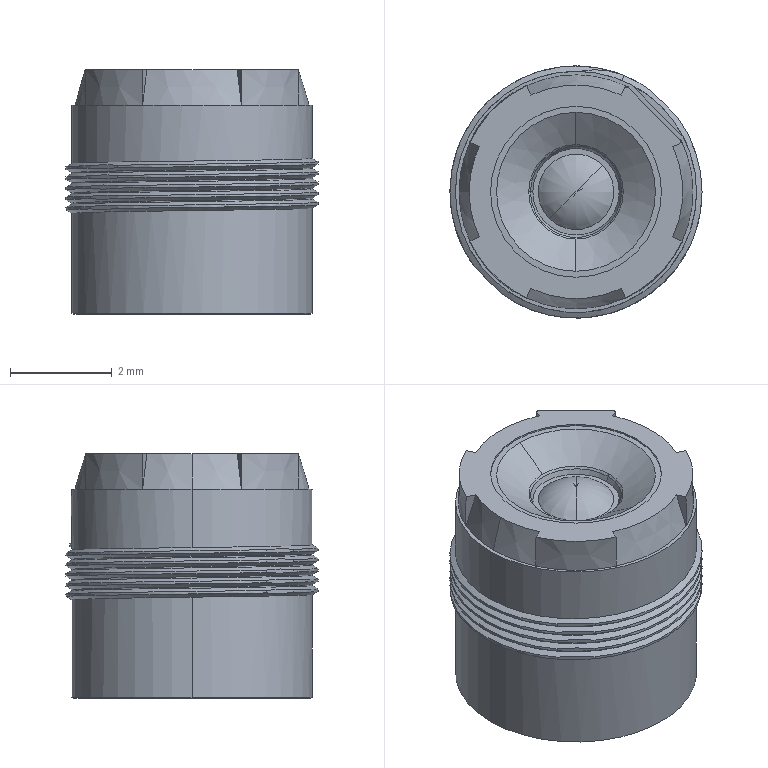Part | SolidWorks | features BaseBody 1 | 1 solid | 105 faces | box 4.957 x 4.957 x 4.8 mm | volume 80.579 mm3 | cylinder 49 | plane 30 | cone 18 | torus 4 | spline 4 | commonest cylinder face diameters 4.957 x15 4.74 x11 0.1 x8 4.309 x3 4.668 x3 3 x2